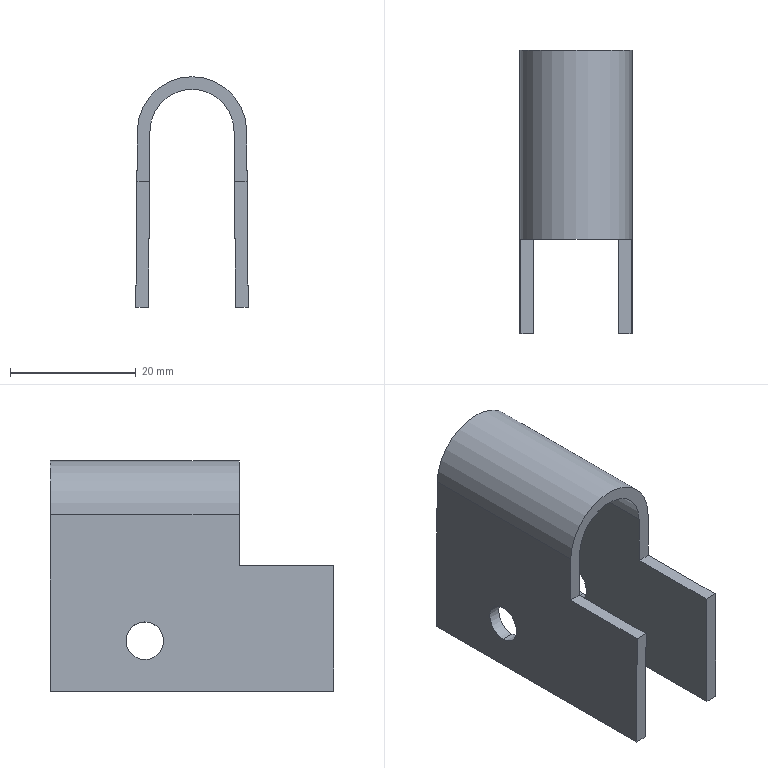Part | SolidWorks | features Bending 1, FlatPattern 1, SMBaseFlange 1, SheetMetal 1 | 1 solid | 18 faces | box 17.852 x 45 x 36.623 mm | volume 5887 mm3 | plane 12 | cylinder 6 | commonest cylinder face diameters 6 x4 13.364 x1 17.364 x1
STEP:
#1=CARTESIAN_POINT('',(-6.883,0.,-31.623));
#2=VERTEX_POINT('',#1);
#3=CARTESIAN_POINT('',(-6.83,0.,-25.623));
#4=VERTEX_POINT('',#3);
#5=CARTESIAN_POINT('',(-6.856,0.,-28.623));
#6=DIRECTION('',(-1.,0.,0.008727));
#7=DIRECTION('',(0.008727,0.,1.));
#8=AXIS2_PLACEMENT_3D('',#5,#6,#7);
#9=CIRCLE('',#8,3.);
#10=EDGE_CURVE('',#2,#4,#9,.T.);
#11=ORIENTED_EDGE('',*,*,#10,.F.);
#12=CARTESIAN_POINT('',(-8.882,0.,-31.605));
#13=VERTEX_POINT('',#12);
#14=CARTESIAN_POINT('',(-6.883,0.,-31.623));
#15=DIRECTION('',(-1.,0.,0.008727));
#16=VECTOR('',#15,1000.);
#17=LINE('',#14,#16);
#18=EDGE_CURVE('',#2,#13,#17,.T.);
#19=ORIENTED_EDGE('',*,*,#18,.T.);
#20=CARTESIAN_POINT('',(-8.83,0.,-25.606));
#21=VERTEX_POINT('',#20);
#22=CARTESIAN_POINT('',(-8.856,0.,-28.606));
#23=DIRECTION('',(-1.,0.,0.008727));
#24=DIRECTION('',(0.008727,0.,1.));
#25=AXIS2_PLACEMENT_3D('',#22,#23,#24);
#26=CIRCLE('',#25,3.);
#27=EDGE_CURVE('',#13,#21,#26,.T.);
#28=ORIENTED_EDGE('',*,*,#27,.T.);
#29=CARTESIAN_POINT('',(-6.83,0.,-25.623));
#30=DIRECTION('',(-1.,0.,0.008727));
#31=VECTOR('',#30,1000.);
#32=LINE('',#29,#31);
#33=EDGE_CURVE('',#4,#21,#32,.T.);
#34=ORIENTED_EDGE('',*,*,#33,.F.);
#35=EDGE_LOOP('',(#11,#19,#28,#34));
#36=FACE_OUTER_BOUND('',#35,.T.);
#37=CARTESIAN_POINT('',(-6.856,0.,-28.623));
#38=DIRECTION('',(-1.,0.,0.008727));
#39=DIRECTION('',(0.008727,0.,1.));
#40=AXIS2_PLACEMENT_3D('',#37,#38,#39);
#41=CYLINDRICAL_SURFACE('',#40,3.);
#42=ADVANCED_FACE('',(#36),#41,.F.);
#43=CARTESIAN_POINT('',(6.83,0.,-25.623));
#44=VERTEX_POINT('',#43);
#45=CARTESIAN_POINT('',(6.883,0.,-31.623));
#46=VERTEX_POINT('',#45);
#47=CARTESIAN_POINT('',(6.856,0.,-28.623));
#48=DIRECTION('',(1.,0.,0.008727));
#49=DIRECTION('',(0.008727,0.,-1.));
#50=AXIS2_PLACEMENT_3D('',#47,#48,#49);
#51=CIRCLE('',#50,3.);
#52=EDGE_CURVE('',#44,#46,#51,.T.);
#53=ORIENTED_EDGE('',*,*,#52,.F.);
#54=CARTESIAN_POINT('',(8.83,0.,-25.606));
#55=VERTEX_POINT('',#54);
#56=CARTESIAN_POINT('',(6.83,0.,-25.623));
#57=DIRECTION('',(1.,0.,0.008727));
#58=VECTOR('',#57,1000.);
#59=LINE('',#56,#58);
#60=EDGE_CURVE('',#44,#55,#59,.T.);
#61=ORIENTED_EDGE('',*,*,#60,.T.);
#62=CARTESIAN_POINT('',(8.882,0.,-31.605));
#63=VERTEX_POINT('',#62);
#64=CARTESIAN_POINT('',(8.856,0.,-28.606));
#65=DIRECTION('',(1.,0.,0.008727));
#66=DIRECTION('',(0.008727,0.,-1.));
#67=AXIS2_PLACEMENT_3D('',#64,#65,#66);
#68=CIRCLE('',#67,3.);
#69=EDGE_CURVE('',#55,#63,#68,.T.);
#70=ORIENTED_EDGE('',*,*,#69,.T.);
#71=CARTESIAN_POINT('',(6.883,0.,-31.623));
#72=DIRECTION('',(1.,0.,0.008727));
#73=VECTOR('',#72,1000.);
#74=LINE('',#71,#73);
#75=EDGE_CURVE('',#46,#63,#74,.T.);
#76=ORIENTED_EDGE('',*,*,#75,.F.);
#77=EDGE_LOOP('',(#53,#61,#70,#76));
#78=FACE_OUTER_BOUND('',#77,.T.);
#79=CARTESIAN_POINT('',(6.856,0.,-28.623));
#80=DIRECTION('',(1.,0.,0.008727));
#81=DIRECTION('',(0.008727,0.,-1.));
#82=AXIS2_PLACEMENT_3D('',#79,#80,#81);
#83=CYLINDRICAL_SURFACE('',#82,3.);
#84=ADVANCED_FACE('',(#78),#83,.F.);
#85=ORIENTED_EDGE('',*,*,#60,.F.);
#86=CARTESIAN_POINT('',(6.856,0.,-28.623));
#87=DIRECTION('',(1.,0.,0.008727));
#88=DIRECTION('',(0.008727,0.,-1.));
#89=AXIS2_PLACEMENT_3D('',#86,#87,#88);
#90=CIRCLE('',#89,3.);
#91=EDGE_CURVE('',#46,#44,#90,.T.);
#92=ORIENTED_EDGE('',*,*,#91,.F.);
#93=ORIENTED_EDGE('',*,*,#75,.T.);
#94=CARTESIAN_POINT('',(8.856,0.,-28.606));
#95=DIRECTION('',(1.,0.,0.008727));
#96=DIRECTION('',(0.008727,0.,-1.));
#97=AXIS2_PLACEMENT_3D('',#94,#95,#96);
#98=CIRCLE('',#97,3.);
#99=EDGE_CURVE('',#63,#55,#98,.T.);
#100=ORIENTED_EDGE('',*,*,#99,.T.);
#101=EDGE_LOOP('',(#85,#92,#93,#100));
#102=FACE_OUTER_BOUND('',#101,.T.);
#103=CARTESIAN_POINT('',(6.856,0.,-28.623));
#104=DIRECTION('',(1.,0.,0.008727));
#105=DIRECTION('',(0.008727,0.,-1.));
#106=AXIS2_PLACEMENT_3D('',#103,#104,#105);
#107=CYLINDRICAL_SURFACE('',#106,3.);
#108=ADVANCED_FACE('',(#102),#107,.F.);
#109=ORIENTED_EDGE('',*,*,#18,.F.);
#110=CARTESIAN_POINT('',(-6.856,0.,-28.623));
#111=DIRECTION('',(-1.,0.,0.008727));
#112=DIRECTION('',(0.008727,0.,1.));
#113=AXIS2_PLACEMENT_3D('',#110,#111,#112);
#114=CIRCLE('',#113,3.);
#115=EDGE_CURVE('',#4,#2,#114,.T.);
#116=ORIENTED_EDGE('',*,*,#115,.F.);
#117=ORIENTED_EDGE('',*,*,#33,.T.);
#118=CARTESIAN_POINT('',(-8.856,0.,-28.606));
#119=DIRECTION('',(-1.,0.,0.008727));
#120=DIRECTION('',(0.008727,0.,1.));
#121=AXIS2_PLACEMENT_3D('',#118,#119,#120);
#122=CIRCLE('',#121,3.);
#123=EDGE_CURVE('',#21,#13,#122,.T.);
#124=ORIENTED_EDGE('',*,*,#123,.T.);
#125=EDGE_LOOP('',(#109,#116,#117,#124));
#126=FACE_OUTER_BOUND('',#125,.T.);
#127=CARTESIAN_POINT('',(-6.856,0.,-28.623));
#128=DIRECTION('',(-1.,0.,0.008727));
#129=DIRECTION('',(0.008727,0.,1.));
#130=AXIS2_PLACEMENT_3D('',#127,#128,#129);
#131=CYLINDRICAL_SURFACE('',#130,3.);
#132=ADVANCED_FACE('',(#126),#131,.F.);
#133=CARTESIAN_POINT('',(6.682,15.,-8.624));
#134=VERTEX_POINT('',#133);
#135=CARTESIAN_POINT('',(-6.682,15.,-8.624));
#136=VERTEX_POINT('',#135);
#137=CARTESIAN_POINT('',(0.,15.,-8.682));
#138=DIRECTION('',(0.,-1.,0.));
#139=DIRECTION('',(0.,0.,1.));
#140=AXIS2_PLACEMENT_3D('',#137,#138,#139);
#141=CIRCLE('',#140,6.682);
#142=EDGE_CURVE('',#134,#136,#141,.T.);
#143=ORIENTED_EDGE('',*,*,#142,.F.);
#144=CARTESIAN_POINT('',(6.682,-15.,-8.624));
#145=VERTEX_POINT('',#144);
#146=CARTESIAN_POINT('',(6.682,0.,-8.624));
#147=DIRECTION('',(0.,-1.,0.));
#148=VECTOR('',#147,1000.);
#149=LINE('',#146,#148);
#150=EDGE_CURVE('',#134,#145,#149,.T.);
#151=ORIENTED_EDGE('',*,*,#150,.T.);
#152=CARTESIAN_POINT('',(-6.682,-15.,-8.624));
#153=VERTEX_POINT('',#152);
#154=CARTESIAN_POINT('',(0.,-15.,-8.682));
#155=DIRECTION('',(0.,1.,0.));
#156=DIRECTION('',(0.,0.,1.));
#157=AXIS2_PLACEMENT_3D('',#154,#155,#156);
#158=CIRCLE('',#157,6.682);
#159=EDGE_CURVE('',#153,#145,#158,.T.);
#160=ORIENTED_EDGE('',*,*,#159,.F.);
#161=CARTESIAN_POINT('',(-6.682,0.,-8.624));
#162=DIRECTION('',(0.,-1.,0.));
#163=VECTOR('',#162,1000.);
#164=LINE('',#161,#163);
#165=EDGE_CURVE('',#136,#153,#164,.T.);
#166=ORIENTED_EDGE('',*,*,#165,.F.);
#167=EDGE_LOOP('',(#143,#151,#160,#166));
#168=FACE_OUTER_BOUND('',#167,.T.);
#169=CARTESIAN_POINT('',(0.,-15.,-8.682));
#170=DIRECTION('',(0.,1.,0.));
#171=DIRECTION('',(1.,0.,0.));
#172=AXIS2_PLACEMENT_3D('',#169,#170,#171);
#173=CYLINDRICAL_SURFACE('',#172,6.682);
#174=ADVANCED_FACE('',(#168),#173,.F.);
#175=CARTESIAN_POINT('',(8.682,15.,-8.606));
#176=VERTEX_POINT('',#175);
#177=CARTESIAN_POINT('',(-8.682,15.,-8.606));
#178=VERTEX_POINT('',#177);
#179=CARTESIAN_POINT('',(0.,15.,-8.682));
#180=DIRECTION('',(0.,-1.,0.));
#181=DIRECTION('',(0.,0.,1.));
#182=AXIS2_PLACEMENT_3D('',#179,#180,#181);
#183=CIRCLE('',#182,8.682);
#184=EDGE_CURVE('',#176,#178,#183,.T.);
#185=ORIENTED_EDGE('',*,*,#184,.F.);
#186=CARTESIAN_POINT('',(8.926,15.,-36.605));
#187=VERTEX_POINT('',#186);
#188=CARTESIAN_POINT('',(8.228,15.,43.392));
#189=DIRECTION('',(-0.008727,0.,1.));
#190=VECTOR('',#189,1000.);
#191=LINE('',#188,#190);
#192=EDGE_CURVE('',#187,#176,#191,.T.);
#193=ORIENTED_EDGE('',*,*,#192,.F.);
#194=CARTESIAN_POINT('',(6.926,15.,-36.623));
#195=VERTEX_POINT('',#194);
#196=CARTESIAN_POINT('',(6.926,15.,-36.623));
#197=DIRECTION('',(1.,0.,0.008727));
#198=VECTOR('',#197,1000.);
#199=LINE('',#196,#198);
#200=EDGE_CURVE('',#195,#187,#199,.T.);
#201=ORIENTED_EDGE('',*,*,#200,.F.);
#202=CARTESIAN_POINT('',(6.228,15.,43.374));
#203=DIRECTION('',(-0.008727,0.,1.));
#204=VECTOR('',#203,1000.);
#205=LINE('',#202,#204);
#206=EDGE_CURVE('',#195,#134,#205,.T.);
#207=ORIENTED_EDGE('',*,*,#206,.T.);
#208=ORIENTED_EDGE('',*,*,#142,.T.);
#209=CARTESIAN_POINT('',(-6.926,15.,-36.623));
#210=VERTEX_POINT('',#209);
#211=CARTESIAN_POINT('',(-6.926,15.,-36.623));
#212=DIRECTION('',(-0.008727,0.,-1.));
#213=VECTOR('',#212,1000.);
#214=LINE('',#211,#213);
#215=EDGE_CURVE('',#136,#210,#214,.T.);
#216=ORIENTED_EDGE('',*,*,#215,.T.);
#217=CARTESIAN_POINT('',(-8.926,15.,-36.605));
#218=VERTEX_POINT('',#217);
#219=CARTESIAN_POINT('',(-6.926,15.,-36.623));
#220=DIRECTION('',(-1.,0.,0.008727));
#221=VECTOR('',#220,1000.);
#222=LINE('',#219,#221);
#223=EDGE_CURVE('',#210,#218,#222,.T.);
#224=ORIENTED_EDGE('',*,*,#223,.T.);
#225=CARTESIAN_POINT('',(-8.926,15.,-36.605));
#226=DIRECTION('',(-0.008727,0.,-1.));
#227=VECTOR('',#226,1000.);
#228=LINE('',#225,#227);
#229=EDGE_CURVE('',#178,#218,#228,.T.);
#230=ORIENTED_EDGE('',*,*,#229,.F.);
#231=EDGE_LOOP('',(#185,#193,#201,#207,#208,#216,#224,#230));
#232=FACE_OUTER_BOUND('',#231,.T.);
#233=CARTESIAN_POINT('',(0.,15.,38.));
#234=DIRECTION('',(0.,1.,0.));
#235=DIRECTION('',(0.,0.,1.));
#236=AXIS2_PLACEMENT_3D('',#233,#234,#235);
#237=PLANE('',#236);
#238=ADVANCED_FACE('',(#232),#237,.T.);
#239=ORIENTED_EDGE('',*,*,#159,.T.);
#240=CARTESIAN_POINT('',(6.752,-15.,-16.623));
#241=VERTEX_POINT('',#240);
#242=CARTESIAN_POINT('',(6.403,-15.,23.375));
#243=DIRECTION('',(0.008727,0.,-1.));
#244=VECTOR('',#243,1000.);
#245=LINE('',#242,#244);
#246=EDGE_CURVE('',#145,#241,#245,.T.);
#247=ORIENTED_EDGE('',*,*,#246,.T.);
#248=CARTESIAN_POINT('',(8.752,-15.,-16.606));
#249=VERTEX_POINT('',#248);
#250=CARTESIAN_POINT('',(6.752,-15.,-16.623));
#251=DIRECTION('',(1.,0.,0.008727));
#252=VECTOR('',#251,1000.);
#253=LINE('',#250,#252);
#254=EDGE_CURVE('',#241,#249,#253,.T.);
#255=ORIENTED_EDGE('',*,*,#254,.T.);
#256=CARTESIAN_POINT('',(8.682,-15.,-8.606));
#257=VERTEX_POINT('',#256);
#258=CARTESIAN_POINT('',(8.403,-15.,23.392));
#259=DIRECTION('',(0.008727,0.,-1.));
#260=VECTOR('',#259,1000.);
#261=LINE('',#258,#260);
#262=EDGE_CURVE('',#257,#249,#261,.T.);
#263=ORIENTED_EDGE('',*,*,#262,.F.);
#264=CARTESIAN_POINT('',(-8.682,-15.,-8.606));
#265=VERTEX_POINT('',#264);
#266=CARTESIAN_POINT('',(0.,-15.,-8.682));
#267=DIRECTION('',(0.,1.,0.));
#268=DIRECTION('',(0.,0.,1.));
#269=AXIS2_PLACEMENT_3D('',#266,#267,#268);
#270=CIRCLE('',#269,8.682);
#271=EDGE_CURVE('',#265,#257,#270,.T.);
#272=ORIENTED_EDGE('',*,*,#271,.F.);
#273=CARTESIAN_POINT('',(-8.752,-15.,-16.606));
#274=VERTEX_POINT('',#273);
#275=CARTESIAN_POINT('',(-8.752,-15.,-16.606));
#276=DIRECTION('',(0.008727,0.,1.));
#277=VECTOR('',#276,1000.);
#278=LINE('',#275,#277);
#279=EDGE_CURVE('',#274,#265,#278,.T.);
#280=ORIENTED_EDGE('',*,*,#279,.F.);
#281=CARTESIAN_POINT('',(-6.752,-15.,-16.623));
#282=VERTEX_POINT('',#281);
#283=CARTESIAN_POINT('',(-6.752,-15.,-16.623));
#284=DIRECTION('',(-1.,0.,0.008727));
#285=VECTOR('',#284,1000.);
#286=LINE('',#283,#285);
#287=EDGE_CURVE('',#282,#274,#286,.T.);
#288=ORIENTED_EDGE('',*,*,#287,.F.);
#289=CARTESIAN_POINT('',(-6.752,-15.,-16.623));
#290=DIRECTION('',(0.008727,0.,1.));
#291=VECTOR('',#290,1000.);
#292=LINE('',#289,#291);
#293=EDGE_CURVE('',#282,#153,#292,.T.);
#294=ORIENTED_EDGE('',*,*,#293,.T.);
#295=EDGE_LOOP('',(#239,#247,#255,#263,#272,#280,#288,#294));
#296=FACE_OUTER_BOUND('',#295,.T.);
#297=CARTESIAN_POINT('',(0.,-15.,18.));
#298=DIRECTION('',(0.,1.,0.));
#299=DIRECTION('',(0.,0.,1.));
#300=AXIS2_PLACEMENT_3D('',#297,#298,#299);
#301=PLANE('',#300);
#302=ADVANCED_FACE('',(#296),#301,.F.);
#303=ORIENTED_EDGE('',*,*,#99,.F.);
#304=ORIENTED_EDGE('',*,*,#69,.F.);
#305=EDGE_LOOP('',(#303,#304));
#306=FACE_BOUND('',#305,.T.);
#307=ORIENTED_EDGE('',*,*,#192,.T.);
#308=CARTESIAN_POINT('',(8.682,0.,-8.606));
#309=DIRECTION('',(0.,-1.,0.));
#310=VECTOR('',#309,1000.);
#311=LINE('',#308,#310);
#312=EDGE_CURVE('',#176,#257,#311,.T.);
#313=ORIENTED_EDGE('',*,*,#312,.T.);
#314=ORIENTED_EDGE('',*,*,#262,.T.);
#315=CARTESIAN_POINT('',(8.752,-30.,-16.606));
#316=VERTEX_POINT('',#315);
#317=CARTESIAN_POINT('',(8.752,-15.,-16.606));
#318=DIRECTION('',(0.,-1.,0.));
#319=VECTOR('',#318,1000.);
#320=LINE('',#317,#319);
#321=EDGE_CURVE('',#249,#316,#320,.T.);
#322=ORIENTED_EDGE('',*,*,#321,.T.);
#323=CARTESIAN_POINT('',(8.926,-30.,-36.605));
#324=VERTEX_POINT('',#323);
#325=CARTESIAN_POINT('',(8.926,-30.,-36.605));
#326=DIRECTION('',(0.008727,0.,-1.));
#327=VECTOR('',#326,1000.);
#328=LINE('',#325,#327);
#329=EDGE_CURVE('',#316,#324,#328,.T.);
#330=ORIENTED_EDGE('',*,*,#329,.T.);
#331=CARTESIAN_POINT('',(8.926,15.,-36.605));
#332=DIRECTION('',(0.,1.,0.));
#333=VECTOR('',#332,1000.);
#334=LINE('',#331,#333);
#335=EDGE_CURVE('',#324,#187,#334,.T.);
#336=ORIENTED_EDGE('',*,*,#335,.T.);
#337=EDGE_LOOP('',(#307,#313,#314,#322,#330,#336));
#338=FACE_OUTER_BOUND('',#337,.T.);
#339=CARTESIAN_POINT('',(8.577,0.,3.393));
#340=DIRECTION('',(-1.,0.,-0.008727));
#341=DIRECTION('',(-0.008727,0.,1.));
#342=AXIS2_PLACEMENT_3D('',#339,#340,#341);
#343=PLANE('',#342);
#344=ADVANCED_FACE('',(#306,#338),#343,.F.);
#345=ORIENTED_EDGE('',*,*,#312,.F.);
#346=ORIENTED_EDGE('',*,*,#184,.T.);
#347=CARTESIAN_POINT('',(-8.682,0.,-8.606));
#348=DIRECTION('',(0.,-1.,0.));
#349=VECTOR('',#348,1000.);
#350=LINE('',#347,#349);
#351=EDGE_CURVE('',#178,#265,#350,.T.);
#352=ORIENTED_EDGE('',*,*,#351,.T.);
#353=ORIENTED_EDGE('',*,*,#271,.T.);
#354=EDGE_LOOP('',(#345,#346,#352,#353));
#355=FACE_OUTER_BOUND('',#354,.T.);
#356=CARTESIAN_POINT('',(0.,-15.,-8.682));
#357=DIRECTION('',(0.,1.,0.));
#358=DIRECTION('',(1.,0.,0.));
#359=AXIS2_PLACEMENT_3D('',#356,#357,#358);
#360=CYLINDRICAL_SURFACE('',#359,8.682);
#361=ADVANCED_FACE('',(#355),#360,.T.);
#362=ORIENTED_EDGE('',*,*,#115,.T.);
#363=ORIENTED_EDGE('',*,*,#10,.T.);
#364=EDGE_LOOP('',(#362,#363));
#365=FACE_BOUND('',#364,.T.);
#366=ORIENTED_EDGE('',*,*,#215,.F.);
#367=ORIENTED_EDGE('',*,*,#165,.T.);
#368=ORIENTED_EDGE('',*,*,#293,.F.);
#369=CARTESIAN_POINT('',(-6.752,-30.,-16.623));
#370=VERTEX_POINT('',#369);
#371=CARTESIAN_POINT('',(-6.752,-15.,-16.623));
#372=DIRECTION('',(0.,1.,0.));
#373=VECTOR('',#372,1000.);
#374=LINE('',#371,#373);
#375=EDGE_CURVE('',#370,#282,#374,.T.);
#376=ORIENTED_EDGE('',*,*,#375,.F.);
#377=CARTESIAN_POINT('',(-6.926,-30.,-36.623));
#378=VERTEX_POINT('',#377);
#379=CARTESIAN_POINT('',(-6.926,-30.,-36.623));
#380=DIRECTION('',(0.008727,0.,1.));
#381=VECTOR('',#380,1000.);
#382=LINE('',#379,#381);
#383=EDGE_CURVE('',#378,#370,#382,.T.);
#384=ORIENTED_EDGE('',*,*,#383,.F.);
#385=CARTESIAN_POINT('',(-6.926,15.,-36.623));
#386=DIRECTION('',(0.,-1.,0.));
#387=VECTOR('',#386,1000.);
#388=LINE('',#385,#387);
#389=EDGE_CURVE('',#210,#378,#388,.T.);
#390=ORIENTED_EDGE('',*,*,#389,.F.);
#391=EDGE_LOOP('',(#366,#367,#368,#376,#384,#390));
#392=FACE_OUTER_BOUND('',#391,.T.);
#393=CARTESIAN_POINT('',(-6.577,0.,3.376));
#394=DIRECTION('',(1.,0.,-0.008727));
#395=DIRECTION('',(-0.008727,0.,-1.));
#396=AXIS2_PLACEMENT_3D('',#393,#394,#395);
#397=PLANE('',#396);
#398=ADVANCED_FACE('',(#365,#392),#397,.T.);
#399=ORIENTED_EDGE('',*,*,#329,.F.);
#400=CARTESIAN_POINT('',(6.752,-30.,-16.623));
#401=VERTEX_POINT('',#400);
#402=CARTESIAN_POINT('',(6.752,-30.,-16.623));
#403=DIRECTION('',(1.,0.,0.008727));
#404=VECTOR('',#403,1000.);
#405=LINE('',#402,#404);
#406=EDGE_CURVE('',#401,#316,#405,.T.);
#407=ORIENTED_EDGE('',*,*,#406,.F.);
#408=CARTESIAN_POINT('',(6.926,-30.,-36.623));
#409=VERTEX_POINT('',#408);
#410=CARTESIAN_POINT('',(6.926,-30.,-36.623));
#411=DIRECTION('',(0.008727,0.,-1.));
#412=VECTOR('',#411,1000.);
#413=LINE('',#410,#412);
#414=EDGE_CURVE('',#401,#409,#413,.T.);
#415=ORIENTED_EDGE('',*,*,#414,.T.);
#416=CARTESIAN_POINT('',(6.926,-30.,-36.623));
#417=DIRECTION('',(1.,0.,0.008727));
#418=VECTOR('',#417,1000.);
#419=LINE('',#416,#418);
#420=EDGE_CURVE('',#409,#324,#419,.T.);
#421=ORIENTED_EDGE('',*,*,#420,.T.);
#422=EDGE_LOOP('',(#399,#407,#415,#421));
#423=FACE_OUTER_BOUND('',#422,.T.);
#424=CARTESIAN_POINT('',(6.926,-30.,-36.623));
#425=DIRECTION('',(0.,-1.,0.));
#426=DIRECTION('',(0.008727,0.,-1.));
#427=AXIS2_PLACEMENT_3D('',#424,#425,#426);
#428=PLANE('',#427);
#429=ADVANCED_FACE('',(#423),#428,.T.);
#430=ORIENTED_EDGE('',*,*,#321,.F.);
#431=ORIENTED_EDGE('',*,*,#254,.F.);
#432=CARTESIAN_POINT('',(6.752,-15.,-16.623));
#433=DIRECTION('',(0.,-1.,0.));
#434=VECTOR('',#433,1000.);
#435=LINE('',#432,#434);
#436=EDGE_CURVE('',#241,#401,#435,.T.);
#437=ORIENTED_EDGE('',*,*,#436,.T.);
#438=ORIENTED_EDGE('',*,*,#406,.T.);
#439=EDGE_LOOP('',(#430,#431,#437,#438));
#440=FACE_OUTER_BOUND('',#439,.T.);
#441=CARTESIAN_POINT('',(6.752,-15.,-16.623));
#442=DIRECTION('',(-0.008727,0.,1.));
#443=DIRECTION('',(0.,-1.,0.));
#444=AXIS2_PLACEMENT_3D('',#441,#442,#443);
#445=PLANE('',#444);
#446=ADVANCED_FACE('',(#440),#445,.T.);
#447=CARTESIAN_POINT('',(-8.752,-30.,-16.606));
#448=VERTEX_POINT('',#447);
#449=CARTESIAN_POINT('',(-8.752,-15.,-16.606));
#450=DIRECTION('',(0.,1.,0.));
#451=VECTOR('',#450,1000.);
#452=LINE('',#449,#451);
#453=EDGE_CURVE('',#448,#274,#452,.T.);
#454=ORIENTED_EDGE('',*,*,#453,.F.);
#455=CARTESIAN_POINT('',(-6.752,-30.,-16.623));
#456=DIRECTION('',(-1.,0.,0.008727));
#457=VECTOR('',#456,1000.);
#458=LINE('',#455,#457);
#459=EDGE_CURVE('',#370,#448,#458,.T.);
#460=ORIENTED_EDGE('',*,*,#459,.F.);
#461=ORIENTED_EDGE('',*,*,#375,.T.);
#462=ORIENTED_EDGE('',*,*,#287,.T.);
#463=EDGE_LOOP('',(#454,#460,#461,#462));
#464=FACE_OUTER_BOUND('',#463,.T.);
#465=CARTESIAN_POINT('',(-6.752,-15.,-16.623));
#466=DIRECTION('',(0.008727,0.,1.));
#467=DIRECTION('',(1.,0.,-0.008727));
#468=AXIS2_PLACEMENT_3D('',#465,#466,#467);
#469=PLANE('',#468);
#470=ADVANCED_FACE('',(#464),#469,.T.);
#471=CARTESIAN_POINT('',(-8.926,-30.,-36.605));
#472=VERTEX_POINT('',#471);
#473=CARTESIAN_POINT('',(-8.926,-30.,-36.605));
#474=DIRECTION('',(0.008727,0.,1.));
#475=VECTOR('',#474,1000.);
#476=LINE('',#473,#475);
#477=EDGE_CURVE('',#472,#448,#476,.T.);
#478=ORIENTED_EDGE('',*,*,#477,.F.);
#479=CARTESIAN_POINT('',(-6.926,-30.,-36.623));
#480=DIRECTION('',(-1.,0.,0.008727));
#481=VECTOR('',#480,1000.);
#482=LINE('',#479,#481);
#483=EDGE_CURVE('',#378,#472,#482,.T.);
#484=ORIENTED_EDGE('',*,*,#483,.F.);
#485=ORIENTED_EDGE('',*,*,#383,.T.);
#486=ORIENTED_EDGE('',*,*,#459,.T.);
#487=EDGE_LOOP('',(#478,#484,#485,#486));
#488=FACE_OUTER_BOUND('',#487,.T.);
#489=CARTESIAN_POINT('',(-6.926,-30.,-36.623));
#490=DIRECTION('',(0.,-1.,0.));
#491=DIRECTION('',(1.,0.,-0.008727));
#492=AXIS2_PLACEMENT_3D('',#489,#490,#491);
#493=PLANE('',#492);
#494=ADVANCED_FACE('',(#488),#493,.T.);
#495=CARTESIAN_POINT('',(-8.926,-15.,-36.605));
#496=DIRECTION('',(0.,-1.,0.));
#497=VECTOR('',#496,1000.);
#498=LINE('',#495,#497);
#499=EDGE_CURVE('',#218,#472,#498,.T.);
#500=ORIENTED_EDGE('',*,*,#499,.F.);
#501=ORIENTED_EDGE('',*,*,#223,.F.);
#502=ORIENTED_EDGE('',*,*,#389,.T.);
#503=ORIENTED_EDGE('',*,*,#483,.T.);
#504=EDGE_LOOP('',(#500,#501,#502,#503));
#505=FACE_OUTER_BOUND('',#504,.T.);
#506=CARTESIAN_POINT('',(-6.926,-15.,-36.623));
#507=DIRECTION('',(-0.008727,0.,-1.));
#508=DIRECTION('',(-1.,0.,0.008727));
#509=AXIS2_PLACEMENT_3D('',#506,#507,#508);
#510=PLANE('',#509);
#511=ADVANCED_FACE('',(#505),#510,.T.);
#512=ORIENTED_EDGE('',*,*,#335,.F.);
#513=ORIENTED_EDGE('',*,*,#420,.F.);
#514=CARTESIAN_POINT('',(6.926,-15.,-36.623));
#515=DIRECTION('',(0.,1.,0.));
#516=VECTOR('',#515,1000.);
#517=LINE('',#514,#516);
#518=EDGE_CURVE('',#409,#195,#517,.T.);
#519=ORIENTED_EDGE('',*,*,#518,.T.);
#520=ORIENTED_EDGE('',*,*,#200,.T.);
#521=EDGE_LOOP('',(#512,#513,#519,#520));
#522=FACE_OUTER_BOUND('',#521,.T.);
#523=CARTESIAN_POINT('',(6.926,15.,-36.623));
#524=DIRECTION('',(0.008727,0.,-1.));
#525=DIRECTION('',(-1.,0.,-0.008727));
#526=AXIS2_PLACEMENT_3D('',#523,#524,#525);
#527=PLANE('',#526);
#528=ADVANCED_FACE('',(#522),#527,.T.);
#529=ORIENTED_EDGE('',*,*,#150,.F.);
#530=ORIENTED_EDGE('',*,*,#206,.F.);
#531=ORIENTED_EDGE('',*,*,#518,.F.);
#532=ORIENTED_EDGE('',*,*,#414,.F.);
#533=ORIENTED_EDGE('',*,*,#436,.F.);
#534=ORIENTED_EDGE('',*,*,#246,.F.);
#535=EDGE_LOOP('',(#529,#530,#531,#532,#533,#534));
#536=FACE_OUTER_BOUND('',#535,.T.);
#537=ORIENTED_EDGE('',*,*,#91,.T.);
#538=ORIENTED_EDGE('',*,*,#52,.T.);
#539=EDGE_LOOP('',(#537,#538));
#540=FACE_BOUND('',#539,.T.);
#541=CARTESIAN_POINT('',(6.577,0.,3.376));
#542=DIRECTION('',(-1.,0.,-0.008727));
#543=DIRECTION('',(-0.008727,0.,1.));
#544=AXIS2_PLACEMENT_3D('',#541,#542,#543);
#545=PLANE('',#544);
#546=ADVANCED_FACE('',(#536,#540),#545,.T.);
#547=ORIENTED_EDGE('',*,*,#351,.F.);
#548=ORIENTED_EDGE('',*,*,#229,.T.);
#549=ORIENTED_EDGE('',*,*,#499,.T.);
#550=ORIENTED_EDGE('',*,*,#477,.T.);
#551=ORIENTED_EDGE('',*,*,#453,.T.);
#552=ORIENTED_EDGE('',*,*,#279,.T.);
#553=EDGE_LOOP('',(#547,#548,#549,#550,#551,#552));
#554=FACE_OUTER_BOUND('',#553,.T.);
#555=ORIENTED_EDGE('',*,*,#123,.F.);
#556=ORIENTED_EDGE('',*,*,#27,.F.);
#557=EDGE_LOOP('',(#555,#556));
#558=FACE_BOUND('',#557,.T.);
#559=CARTESIAN_POINT('',(-8.577,0.,3.393));
#560=DIRECTION('',(1.,0.,-0.008727));
#561=DIRECTION('',(-0.008727,0.,-1.));
#562=AXIS2_PLACEMENT_3D('',#559,#560,#561);
#563=PLANE('',#562);
#564=ADVANCED_FACE('',(#554,#558),#563,.F.);
#565=CLOSED_SHELL('',(#42,#84,#108,#132,#174,#238,#302,#344,#361,#398,#429,#446,#470,#494,#511,#528,#546,#564));
#566=MANIFOLD_SOLID_BREP('',#565);
#567=CARTESIAN_POINT('',(0.,0.,0.));
#568=DIRECTION('',(0.,0.,1.));
#569=DIRECTION('',(1.,0.,0.));
#570=AXIS2_PLACEMENT_3D('',#567,#568,#569);
#571=(LENGTH_UNIT()NAMED_UNIT(*)SI_UNIT(.MILLI.,.METRE.));
#572=UNCERTAINTY_MEASURE_WITH_UNIT(LENGTH_MEASURE(0.00001),#571,'','');
#573=(NAMED_UNIT(*)PLANE_ANGLE_UNIT()SI_UNIT($,.RADIAN.));
#574=(NAMED_UNIT(*)SI_UNIT($,.STERADIAN.)SOLID_ANGLE_UNIT());
#575=(GEOMETRIC_REPRESENTATION_CONTEXT(3)GLOBAL_UNCERTAINTY_ASSIGNED_CONTEXT((#572))GLOBAL_UNIT_ASSIGNED_CONTEXT((#571,#573,#574))REPRESENTATION_CONTEXT('',''));
#576=ADVANCED_BREP_SHAPE_REPRESENTATION('',(#566,#570),#575);